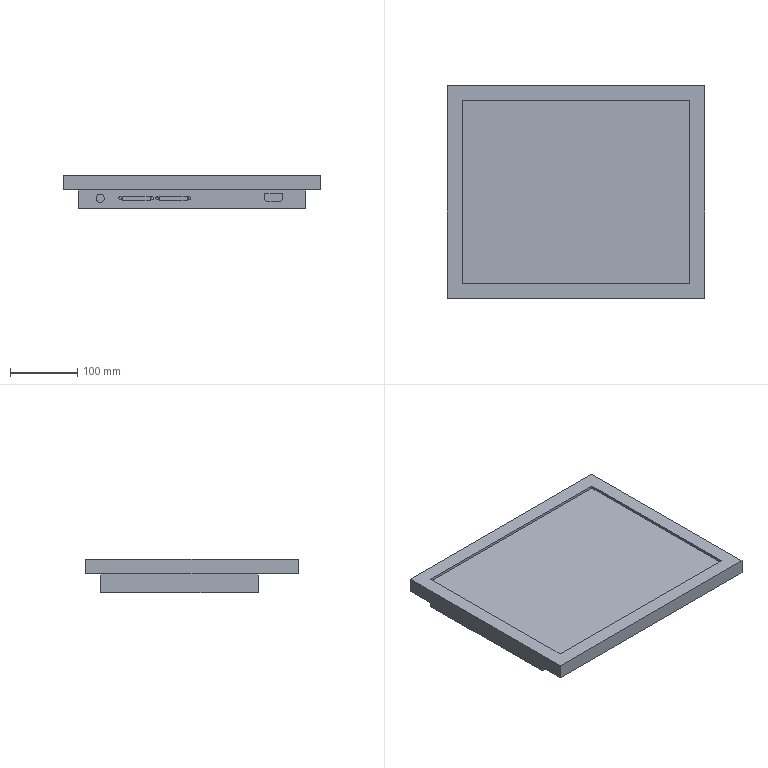Part | SolidWorks | features ICE 2, Chamfer 1, CutThin 1, Extrusion 1, HoleWzd 1, MoveFace 1 | 1 solid | 64 faces | box 384 x 316.5 x 50 mm | volume 4529826 mm3 | plane 38 | cylinder 18 | cone 8 | commonest cylinder face diameters 4.2 x16 12 x2